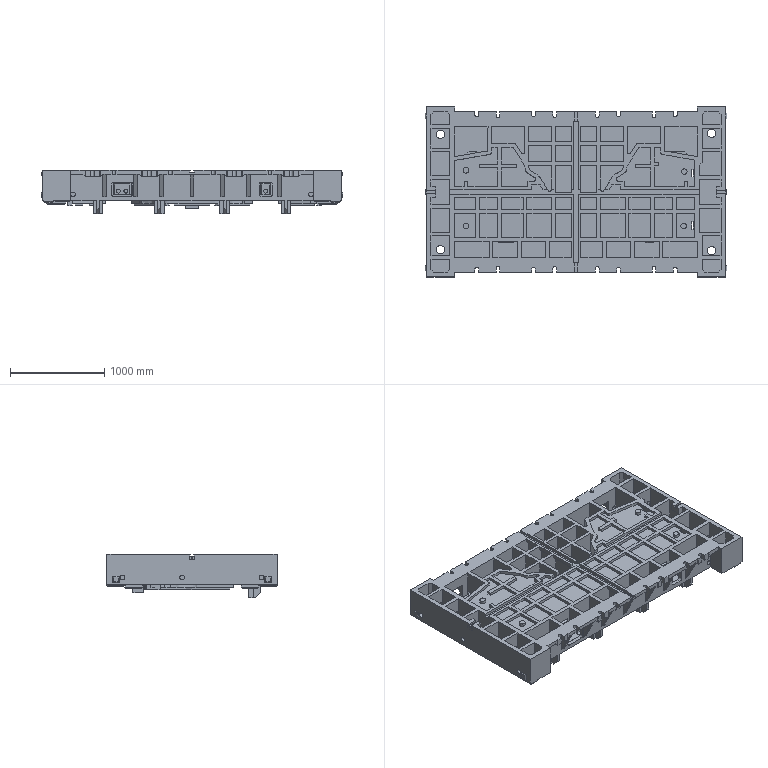Part | NX | features solid 2 | 1 solid | 1304 faces | box 3190 x 1800 x 460 mm | volume 625663920 mm3 | plane 1085 | cylinder 154 | spline 65 | commonest cylinder face diameters 50 x44 40 x41 60 x26 20 x11 80 x8 42 x6